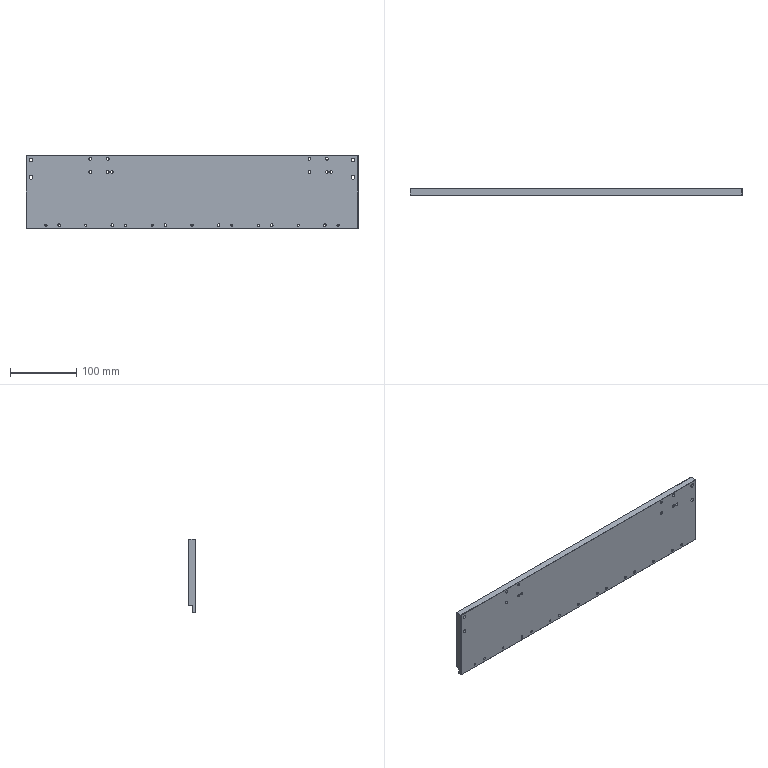Part | NX | 1 solid | 139 faces | box 500 x 10 x 110 mm | volume 518625 mm3 | cone 58 | cylinder 58 | plane 23 | commonest cylinder face diameters 3.3 x18 4 x16 4.2 x16 5.5 x8